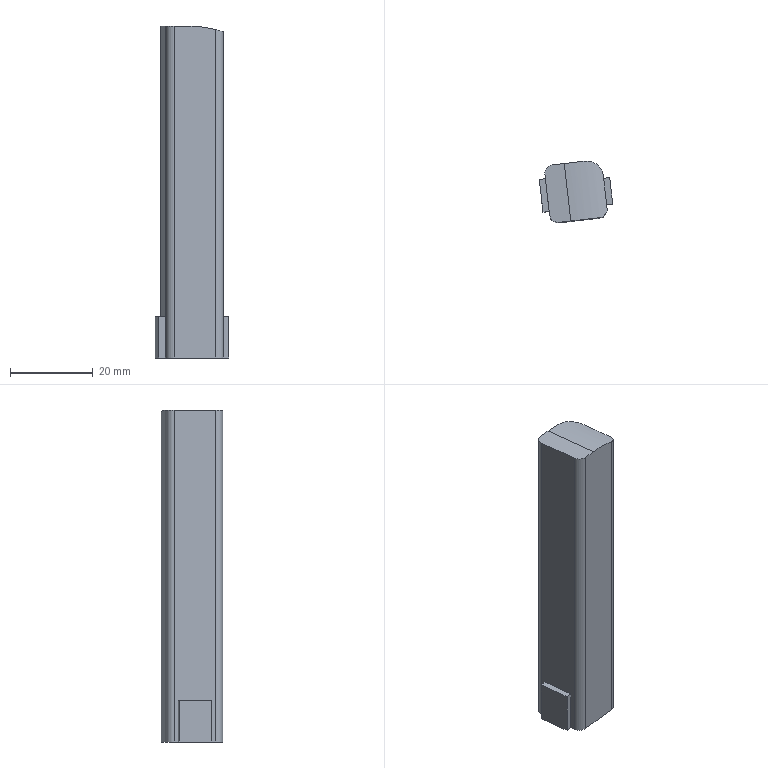Part | NX | features solid 2 | 1 solid | 19 faces | box 17.796 x 14.854 x 80.4 mm | volume 15437 mm3 | plane 14 | cylinder 5 | commonest cylinder face diameters 4 x3 8 x1 59 x1
STEP:
#1=CARTESIAN_POINT('',(2069.672,191.776,-68.));
#2=VERTEX_POINT('',#1);
#3=CARTESIAN_POINT('',(2070.408,185.318,-68.));
#4=VERTEX_POINT('',#3);
#5=CARTESIAN_POINT('',(2069.955,189.292,-68.));
#6=DIRECTION('',(0.1132,-0.9936,0.));
#7=VECTOR('',#6,1000.);
#8=LINE('',#5,#7);
#9=EDGE_CURVE('',#2,#4,#8,.T.);
#10=ORIENTED_EDGE('',*,*,#9,.F.);
#11=CARTESIAN_POINT('',(2069.672,191.776,-78.));
#12=VERTEX_POINT('',#11);
#13=CARTESIAN_POINT('',(2069.672,191.776,-63.));
#14=DIRECTION('',(0.,0.,-1.));
#15=VECTOR('',#14,1000.);
#16=LINE('',#13,#15);
#17=EDGE_CURVE('',#2,#12,#16,.T.);
#18=ORIENTED_EDGE('',*,*,#17,.T.);
#19=CARTESIAN_POINT('',(2069.615,192.273,-78.));
#20=VERTEX_POINT('',#19);
#21=CARTESIAN_POINT('',(2069.955,189.292,-78.));
#22=DIRECTION('',(0.1132,-0.9936,0.));
#23=VECTOR('',#22,1000.);
#24=LINE('',#21,#23);
#25=EDGE_CURVE('',#20,#12,#24,.T.);
#26=ORIENTED_EDGE('',*,*,#25,.F.);
#27=CARTESIAN_POINT('',(2069.615,192.273,0.9709));
#28=VERTEX_POINT('',#27);
#29=CARTESIAN_POINT('',(2069.615,192.273,-63.));
#30=DIRECTION('',(0.,0.,-1.));
#31=VECTOR('',#30,1000.);
#32=LINE('',#29,#31);
#33=EDGE_CURVE('',#28,#20,#32,.T.);
#34=ORIENTED_EDGE('',*,*,#33,.F.);
#35=CARTESIAN_POINT('',(2070.521,184.325,0.9709));
#36=VERTEX_POINT('',#35);
#37=CARTESIAN_POINT('',(2070.521,184.325,0.9709));
#38=CARTESIAN_POINT('',(2070.219,186.974,0.9709));
#39=CARTESIAN_POINT('',(2069.917,189.624,0.9709));
#40=CARTESIAN_POINT('',(2069.615,192.273,0.9709));
#41=B_SPLINE_CURVE_WITH_KNOTS('',3,(#37,#38,#39,#40),.UNSPECIFIED.,.F.,.F.,(4,4),(0.,1.),.PIECEWISE_BEZIER_KNOTS.);
#42=EDGE_CURVE('',#36,#28,#41,.T.);
#43=ORIENTED_EDGE('',*,*,#42,.F.);
#44=CARTESIAN_POINT('',(2070.521,184.325,-78.));
#45=VERTEX_POINT('',#44);
#46=CARTESIAN_POINT('',(2070.521,184.325,-63.));
#47=DIRECTION('',(0.,0.,-1.));
#48=VECTOR('',#47,1000.);
#49=LINE('',#46,#48);
#50=EDGE_CURVE('',#36,#45,#49,.T.);
#51=ORIENTED_EDGE('',*,*,#50,.T.);
#52=CARTESIAN_POINT('',(2070.408,185.318,-78.));
#53=VERTEX_POINT('',#52);
#54=CARTESIAN_POINT('',(2069.955,189.292,-78.));
#55=DIRECTION('',(0.1132,-0.9936,0.));
#56=VECTOR('',#55,1000.);
#57=LINE('',#54,#56);
#58=EDGE_CURVE('',#53,#45,#57,.T.);
#59=ORIENTED_EDGE('',*,*,#58,.F.);
#60=CARTESIAN_POINT('',(2070.408,185.318,-63.));
#61=DIRECTION('',(0.,0.,-1.));
#62=VECTOR('',#61,1000.);
#63=LINE('',#60,#62);
#64=EDGE_CURVE('',#4,#53,#63,.T.);
#65=ORIENTED_EDGE('',*,*,#64,.F.);
#66=EDGE_LOOP('',(#10,#18,#26,#34,#43,#51,#59,#65));
#67=FACE_BOUND('',#66,.T.);
#68=CARTESIAN_POINT('',(2069.955,189.292,-63.));
#69=DIRECTION('',(0.9936,0.1132,0.));
#70=DIRECTION('',(0.,0.,1.));
#71=AXIS2_PLACEMENT_3D('',#68,#69,#70);
#72=PLANE('',#71);
#73=ADVANCED_FACE('',(#67),#72,.T.);
#74=CARTESIAN_POINT('',(2056.498,183.733,-68.));
#75=VERTEX_POINT('',#74);
#76=CARTESIAN_POINT('',(2055.592,191.682,-68.));
#77=VERTEX_POINT('',#76);
#78=CARTESIAN_POINT('',(2056.045,187.708,-68.));
#79=DIRECTION('',(-0.1132,0.9936,0.));
#80=VECTOR('',#79,1000.);
#81=LINE('',#78,#80);
#82=EDGE_CURVE('',#75,#77,#81,.T.);
#83=ORIENTED_EDGE('',*,*,#82,.F.);
#84=CARTESIAN_POINT('',(2056.498,183.733,-78.));
#85=VERTEX_POINT('',#84);
#86=CARTESIAN_POINT('',(2056.498,183.733,-63.));
#87=DIRECTION('',(0.,0.,-1.));
#88=VECTOR('',#87,1000.);
#89=LINE('',#86,#88);
#90=EDGE_CURVE('',#75,#85,#89,.T.);
#91=ORIENTED_EDGE('',*,*,#90,.T.);
#92=CARTESIAN_POINT('',(2056.611,182.74,-78.));
#93=VERTEX_POINT('',#92);
#94=CARTESIAN_POINT('',(2056.045,187.708,-78.));
#95=DIRECTION('',(-0.1132,0.9936,0.));
#96=VECTOR('',#95,1000.);
#97=LINE('',#94,#96);
#98=EDGE_CURVE('',#93,#85,#97,.T.);
#99=ORIENTED_EDGE('',*,*,#98,.F.);
#100=CARTESIAN_POINT('',(2056.611,182.74,2.4));
#101=VERTEX_POINT('',#100);
#102=CARTESIAN_POINT('',(2056.611,182.74,-63.));
#103=DIRECTION('',(0.,0.,-1.));
#104=VECTOR('',#103,1000.);
#105=LINE('',#102,#104);
#106=EDGE_CURVE('',#101,#93,#105,.T.);
#107=ORIENTED_EDGE('',*,*,#106,.F.);
#108=CARTESIAN_POINT('',(2055.479,192.675,2.4));
#109=VERTEX_POINT('',#108);
#110=CARTESIAN_POINT('',(1900.081,1556.526,2.4));
#111=DIRECTION('',(0.1132,-0.9936,0.000000004));
#112=VECTOR('',#111,1000.);
#113=LINE('',#110,#112);
#114=EDGE_CURVE('',#109,#101,#113,.T.);
#115=ORIENTED_EDGE('',*,*,#114,.F.);
#116=CARTESIAN_POINT('',(2055.479,192.675,-78.));
#117=VERTEX_POINT('',#116);
#118=CARTESIAN_POINT('',(2055.479,192.675,-63.));
#119=DIRECTION('',(0.,0.,-1.));
#120=VECTOR('',#119,1000.);
#121=LINE('',#118,#120);
#122=EDGE_CURVE('',#109,#117,#121,.T.);
#123=ORIENTED_EDGE('',*,*,#122,.T.);
#124=CARTESIAN_POINT('',(2055.592,191.682,-78.));
#125=VERTEX_POINT('',#124);
#126=CARTESIAN_POINT('',(2056.045,187.708,-78.));
#127=DIRECTION('',(-0.1132,0.9936,0.));
#128=VECTOR('',#127,1000.);
#129=LINE('',#126,#128);
#130=EDGE_CURVE('',#125,#117,#129,.T.);
#131=ORIENTED_EDGE('',*,*,#130,.F.);
#132=CARTESIAN_POINT('',(2055.592,191.682,-63.));
#133=DIRECTION('',(0.,0.,-1.));
#134=VECTOR('',#133,1000.);
#135=LINE('',#132,#134);
#136=EDGE_CURVE('',#77,#125,#135,.T.);
#137=ORIENTED_EDGE('',*,*,#136,.F.);
#138=EDGE_LOOP('',(#83,#91,#99,#107,#115,#123,#131,#137));
#139=FACE_BOUND('',#138,.T.);
#140=CARTESIAN_POINT('',(2056.045,187.708,-63.));
#141=DIRECTION('',(-0.9936,-0.1132,0.));
#142=DIRECTION('',(0.,0.,-1.));
#143=AXIS2_PLACEMENT_3D('',#140,#141,#142);
#144=PLANE('',#143);
#145=ADVANCED_FACE('',(#139),#144,.T.);
#146=CARTESIAN_POINT('',(2058.825,180.979,2.4));
#147=VERTEX_POINT('',#146);
#148=CARTESIAN_POINT('',(2058.825,180.979,-78.));
#149=VERTEX_POINT('',#148);
#150=CARTESIAN_POINT('',(2058.825,180.979,-63.));
#151=DIRECTION('',(0.,0.,-1.));
#152=VECTOR('',#151,1000.);
#153=LINE('',#150,#152);
#154=EDGE_CURVE('',#147,#149,#153,.T.);
#155=ORIENTED_EDGE('',*,*,#154,.T.);
#156=CARTESIAN_POINT('',(2068.76,182.111,-78.));
#157=VERTEX_POINT('',#156);
#158=CARTESIAN_POINT('',(2063.792,181.545,-78.));
#159=DIRECTION('',(0.9936,0.1132,0.));
#160=VECTOR('',#159,1000.);
#161=LINE('',#158,#160);
#162=EDGE_CURVE('',#149,#157,#161,.T.);
#163=ORIENTED_EDGE('',*,*,#162,.T.);
#164=CARTESIAN_POINT('',(2068.76,182.111,1.54));
#165=VERTEX_POINT('',#164);
#166=CARTESIAN_POINT('',(2068.76,182.111,-63.));
#167=DIRECTION('',(0.,0.,-1.));
#168=VECTOR('',#167,1000.);
#169=LINE('',#166,#168);
#170=EDGE_CURVE('',#165,#157,#169,.T.);
#171=ORIENTED_EDGE('',*,*,#170,.F.);
#172=CARTESIAN_POINT('',(2061.735,181.311,2.4));
#173=VERTEX_POINT('',#172);
#174=CARTESIAN_POINT('',(2061.735,181.311,-27.1));
#175=DIRECTION('',(-0.1132,0.9936,0.));
#176=DIRECTION('',(-0.9936,-0.1132,0.00081));
#177=AXIS2_PLACEMENT_3D('',#174,#175,#176);
#178=ELLIPSE('',#177,29.5,29.5);
#179=EDGE_CURVE('',#173,#165,#178,.T.);
#180=ORIENTED_EDGE('',*,*,#179,.F.);
#181=CARTESIAN_POINT('',(1280.574,92.305,2.4));
#182=DIRECTION('',(0.9936,0.1132,-0.000000001));
#183=VECTOR('',#182,1000.);
#184=LINE('',#181,#183);
#185=EDGE_CURVE('',#147,#173,#184,.T.);
#186=ORIENTED_EDGE('',*,*,#185,.F.);
#187=EDGE_LOOP('',(#155,#163,#171,#180,#186));
#188=FACE_BOUND('',#187,.T.);
#189=CARTESIAN_POINT('',(2063.792,181.545,-63.));
#190=DIRECTION('',(0.1132,-0.9936,0.));
#191=DIRECTION('',(0.,0.,1.));
#192=AXIS2_PLACEMENT_3D('',#189,#190,#191);
#193=PLANE('',#192);
#194=ADVANCED_FACE('',(#188),#193,.T.);
#195=CARTESIAN_POINT('',(2065.188,195.795,1.961));
#196=VERTEX_POINT('',#195);
#197=CARTESIAN_POINT('',(2065.188,195.795,-78.));
#198=VERTEX_POINT('',#197);
#199=CARTESIAN_POINT('',(2065.188,195.795,-63.));
#200=DIRECTION('',(0.,0.,-1.));
#201=VECTOR('',#200,1000.);
#202=LINE('',#199,#201);
#203=EDGE_CURVE('',#196,#198,#202,.T.);
#204=ORIENTED_EDGE('',*,*,#203,.T.);
#205=CARTESIAN_POINT('',(2057.24,194.889,-78.));
#206=VERTEX_POINT('',#205);
#207=CARTESIAN_POINT('',(2062.208,195.455,-78.));
#208=DIRECTION('',(-0.9936,-0.1132,0.));
#209=VECTOR('',#208,1000.);
#210=LINE('',#207,#209);
#211=EDGE_CURVE('',#198,#206,#210,.T.);
#212=ORIENTED_EDGE('',*,*,#211,.T.);
#213=CARTESIAN_POINT('',(2057.24,194.889,2.4));
#214=VERTEX_POINT('',#213);
#215=CARTESIAN_POINT('',(2057.24,194.889,-63.));
#216=DIRECTION('',(0.,0.,-1.));
#217=VECTOR('',#216,1000.);
#218=LINE('',#215,#217);
#219=EDGE_CURVE('',#214,#206,#218,.T.);
#220=ORIENTED_EDGE('',*,*,#219,.F.);
#221=CARTESIAN_POINT('',(2060.15,195.221,2.4));
#222=VERTEX_POINT('',#221);
#223=CARTESIAN_POINT('',(1278.989,106.215,2.4));
#224=DIRECTION('',(0.9936,0.1132,-0.000000001));
#225=VECTOR('',#224,1000.);
#226=LINE('',#223,#225);
#227=EDGE_CURVE('',#214,#222,#226,.T.);
#228=ORIENTED_EDGE('',*,*,#227,.T.);
#229=CARTESIAN_POINT('',(2060.15,195.221,-27.1));
#230=DIRECTION('',(-0.1132,0.9936,0.));
#231=DIRECTION('',(-0.9936,-0.1132,0.00081));
#232=AXIS2_PLACEMENT_3D('',#229,#230,#231);
#233=ELLIPSE('',#232,29.5,29.5);
#234=EDGE_CURVE('',#222,#196,#233,.T.);
#235=ORIENTED_EDGE('',*,*,#234,.T.);
#236=EDGE_LOOP('',(#204,#212,#220,#228,#235));
#237=FACE_BOUND('',#236,.T.);
#238=CARTESIAN_POINT('',(2062.208,195.455,-63.));
#239=DIRECTION('',(-0.1132,0.9936,0.));
#240=DIRECTION('',(0.,0.,-1.));
#241=AXIS2_PLACEMENT_3D('',#238,#239,#240);
#242=PLANE('',#241);
#243=ADVANCED_FACE('',(#237),#242,.T.);
#244=CARTESIAN_POINT('',(2058.598,182.966,-78.));
#245=DIRECTION('',(0.,0.,-1.));
#246=DIRECTION('',(-1.,0.,0.));
#247=AXIS2_PLACEMENT_3D('',#244,#245,#246);
#248=CIRCLE('',#247,2.);
#249=EDGE_CURVE('',#149,#93,#248,.T.);
#250=ORIENTED_EDGE('',*,*,#249,.F.);
#251=ORIENTED_EDGE('',*,*,#154,.F.);
#252=CARTESIAN_POINT('',(2058.598,182.966,2.4));
#253=DIRECTION('',(0.,-0.000000004,-1.));
#254=DIRECTION('',(0.,1.,-0.000000004));
#255=AXIS2_PLACEMENT_3D('',#252,#253,#254);
#256=CIRCLE('',#255,2.);
#257=EDGE_CURVE('',#147,#101,#256,.T.);
#258=ORIENTED_EDGE('',*,*,#257,.T.);
#259=ORIENTED_EDGE('',*,*,#106,.T.);
#260=EDGE_LOOP('',(#250,#251,#258,#259));
#261=FACE_BOUND('',#260,.T.);
#262=CARTESIAN_POINT('',(2058.598,182.966,-63.));
#263=DIRECTION('',(0.,0.,1.));
#264=DIRECTION('',(-0.9936,-0.1132,0.));
#265=AXIS2_PLACEMENT_3D('',#262,#263,#264);
#266=CYLINDRICAL_SURFACE('',#265,2.);
#267=ADVANCED_FACE('',(#261),#266,.T.);
#268=CARTESIAN_POINT('',(2068.534,184.098,-78.));
#269=DIRECTION('',(0.,0.,-1.));
#270=DIRECTION('',(-1.,0.,0.));
#271=AXIS2_PLACEMENT_3D('',#268,#269,#270);
#272=CIRCLE('',#271,2.);
#273=EDGE_CURVE('',#45,#157,#272,.T.);
#274=ORIENTED_EDGE('',*,*,#273,.F.);
#275=ORIENTED_EDGE('',*,*,#50,.F.);
#276=CARTESIAN_POINT('',(2070.521,184.325,0.9709));
#277=CARTESIAN_POINT('',(2070.643,183.254,0.9709));
#278=CARTESIAN_POINT('',(2069.798,182.229,1.282));
#279=CARTESIAN_POINT('',(2068.76,182.111,1.54));
#280=B_SPLINE_CURVE_WITH_KNOTS('',3,(#276,#277,#278,#279),.UNSPECIFIED.,.F.,.F.,(4,4),(0.,0.003185),.UNSPECIFIED.);
#281=EDGE_CURVE('',#36,#165,#280,.T.);
#282=ORIENTED_EDGE('',*,*,#281,.T.);
#283=ORIENTED_EDGE('',*,*,#170,.T.);
#284=EDGE_LOOP('',(#274,#275,#282,#283));
#285=FACE_BOUND('',#284,.T.);
#286=CARTESIAN_POINT('',(2068.534,184.098,-63.));
#287=DIRECTION('',(0.,0.,1.));
#288=DIRECTION('',(-0.9936,-0.1132,0.));
#289=AXIS2_PLACEMENT_3D('',#286,#287,#288);
#290=CYLINDRICAL_SURFACE('',#289,2.);
#291=ADVANCED_FACE('',(#285),#290,.T.);
#292=CARTESIAN_POINT('',(2065.641,191.82,-78.));
#293=DIRECTION('',(0.,0.,-1.));
#294=DIRECTION('',(-1.,0.,0.));
#295=AXIS2_PLACEMENT_3D('',#292,#293,#294);
#296=CIRCLE('',#295,4.);
#297=EDGE_CURVE('',#198,#20,#296,.T.);
#298=ORIENTED_EDGE('',*,*,#297,.F.);
#299=ORIENTED_EDGE('',*,*,#203,.F.);
#300=CARTESIAN_POINT('',(2069.615,192.273,0.9709));
#301=CARTESIAN_POINT('',(2069.494,193.338,0.9709));
#302=CARTESIAN_POINT('',(2068.368,195.298,1.279));
#303=CARTESIAN_POINT('',(2066.237,195.914,1.777));
#304=CARTESIAN_POINT('',(2065.188,195.795,1.961));
#305=B_SPLINE_CURVE_WITH_KNOTS('',3,(#300,#301,#302,#303,#304),.UNSPECIFIED.,.F.,.F.,(4,1,4),(0.,0.003169,0.006337),.UNSPECIFIED.);
#306=EDGE_CURVE('',#28,#196,#305,.T.);
#307=ORIENTED_EDGE('',*,*,#306,.F.);
#308=ORIENTED_EDGE('',*,*,#33,.T.);
#309=EDGE_LOOP('',(#298,#299,#307,#308));
#310=FACE_BOUND('',#309,.T.);
#311=CARTESIAN_POINT('',(2065.641,191.82,-63.));
#312=DIRECTION('',(0.,0.,-1.));
#313=DIRECTION('',(1.,0.,0.));
#314=AXIS2_PLACEMENT_3D('',#311,#312,#313);
#315=CYLINDRICAL_SURFACE('',#314,4.);
#316=ADVANCED_FACE('',(#310),#315,.T.);
#317=CARTESIAN_POINT('',(2057.466,192.902,-78.));
#318=DIRECTION('',(0.,0.,-1.));
#319=DIRECTION('',(-1.,0.,0.));
#320=AXIS2_PLACEMENT_3D('',#317,#318,#319);
#321=CIRCLE('',#320,2.);
#322=EDGE_CURVE('',#117,#206,#321,.T.);
#323=ORIENTED_EDGE('',*,*,#322,.F.);
#324=ORIENTED_EDGE('',*,*,#122,.F.);
#325=CARTESIAN_POINT('',(2057.466,192.902,2.4));
#326=DIRECTION('',(0.,0.000000004,1.));
#327=DIRECTION('',(0.,1.,-0.000000004));
#328=AXIS2_PLACEMENT_3D('',#325,#326,#327);
#329=CIRCLE('',#328,2.);
#330=EDGE_CURVE('',#214,#109,#329,.T.);
#331=ORIENTED_EDGE('',*,*,#330,.F.);
#332=ORIENTED_EDGE('',*,*,#219,.T.);
#333=EDGE_LOOP('',(#323,#324,#331,#332));
#334=FACE_BOUND('',#333,.T.);
#335=CARTESIAN_POINT('',(2057.466,192.902,-63.));
#336=DIRECTION('',(0.,0.,1.));
#337=DIRECTION('',(-0.9936,-0.1132,0.));
#338=AXIS2_PLACEMENT_3D('',#335,#336,#337);
#339=CYLINDRICAL_SURFACE('',#338,2.);
#340=ADVANCED_FACE('',(#334),#339,.T.);
#341=ORIENTED_EDGE('',*,*,#297,.T.);
#342=ORIENTED_EDGE('',*,*,#25,.T.);
#343=CARTESIAN_POINT('',(2071.162,191.946,-78.));
#344=VERTEX_POINT('',#343);
#345=CARTESIAN_POINT('',(2070.666,191.89,-78.));
#346=DIRECTION('',(-0.9936,-0.1132,0.));
#347=VECTOR('',#346,1000.);
#348=LINE('',#345,#347);
#349=EDGE_CURVE('',#344,#12,#348,.T.);
#350=ORIENTED_EDGE('',*,*,#349,.F.);
#351=CARTESIAN_POINT('',(2071.898,185.488,-78.));
#352=VERTEX_POINT('',#351);
#353=CARTESIAN_POINT('',(2071.445,189.462,-78.));
#354=DIRECTION('',(0.1132,-0.9936,0.));
#355=VECTOR('',#354,1000.);
#356=LINE('',#353,#355);
#357=EDGE_CURVE('',#344,#352,#356,.T.);
#358=ORIENTED_EDGE('',*,*,#357,.T.);
#359=CARTESIAN_POINT('',(2071.401,185.431,-78.));
#360=DIRECTION('',(-0.9936,-0.1132,0.));
#361=VECTOR('',#360,1000.);
#362=LINE('',#359,#361);
#363=EDGE_CURVE('',#352,#53,#362,.T.);
#364=ORIENTED_EDGE('',*,*,#363,.T.);
#365=ORIENTED_EDGE('',*,*,#58,.T.);
#366=ORIENTED_EDGE('',*,*,#273,.T.);
#367=ORIENTED_EDGE('',*,*,#162,.F.);
#368=ORIENTED_EDGE('',*,*,#249,.T.);
#369=ORIENTED_EDGE('',*,*,#98,.T.);
#370=CARTESIAN_POINT('',(2055.007,183.563,-78.));
#371=VERTEX_POINT('',#370);
#372=CARTESIAN_POINT('',(2055.504,183.62,-78.));
#373=DIRECTION('',(0.9936,0.1132,0.));
#374=VECTOR('',#373,1000.);
#375=LINE('',#372,#374);
#376=EDGE_CURVE('',#371,#85,#375,.T.);
#377=ORIENTED_EDGE('',*,*,#376,.F.);
#378=CARTESIAN_POINT('',(2054.102,191.512,-78.));
#379=VERTEX_POINT('',#378);
#380=CARTESIAN_POINT('',(2054.555,187.538,-78.));
#381=DIRECTION('',(-0.1132,0.9936,0.));
#382=VECTOR('',#381,1000.);
#383=LINE('',#380,#382);
#384=EDGE_CURVE('',#371,#379,#383,.T.);
#385=ORIENTED_EDGE('',*,*,#384,.T.);
#386=CARTESIAN_POINT('',(2054.599,191.569,-78.));
#387=DIRECTION('',(0.9936,0.1132,0.));
#388=VECTOR('',#387,1000.);
#389=LINE('',#386,#388);
#390=EDGE_CURVE('',#379,#125,#389,.T.);
#391=ORIENTED_EDGE('',*,*,#390,.T.);
#392=ORIENTED_EDGE('',*,*,#130,.T.);
#393=ORIENTED_EDGE('',*,*,#322,.T.);
#394=ORIENTED_EDGE('',*,*,#211,.F.);
#395=EDGE_LOOP('',(#341,#342,#350,#358,#364,#365,#366,#367,#368,#369,#377,#385,#391,#392,#393,#394));
#396=FACE_BOUND('',#395,.T.);
#397=CARTESIAN_POINT('',(2063.,188.5,-78.));
#398=DIRECTION('',(0.,0.,-1.));
#399=DIRECTION('',(0.9936,0.1132,0.));
#400=AXIS2_PLACEMENT_3D('',#397,#398,#399);
#401=PLANE('',#400);
#402=ADVANCED_FACE('',(#396),#401,.T.);
#403=ORIENTED_EDGE('',*,*,#257,.F.);
#404=ORIENTED_EDGE('',*,*,#185,.T.);
#405=CARTESIAN_POINT('',(2060.943,188.266,2.4));
#406=DIRECTION('',(-0.1132,0.9936,-0.000000004));
#407=VECTOR('',#406,1000.);
#408=LINE('',#405,#407);
#409=EDGE_CURVE('',#173,#222,#408,.T.);
#410=ORIENTED_EDGE('',*,*,#409,.T.);
#411=ORIENTED_EDGE('',*,*,#227,.F.);
#412=ORIENTED_EDGE('',*,*,#330,.T.);
#413=ORIENTED_EDGE('',*,*,#114,.T.);
#414=EDGE_LOOP('',(#403,#404,#410,#411,#412,#413));
#415=FACE_BOUND('',#414,.T.);
#416=CARTESIAN_POINT('',(1123.818,1468.078,2.4));
#417=DIRECTION('',(0.,-0.000000004,-1.));
#418=DIRECTION('',(-0.09584,-0.9954,0.000000004));
#419=AXIS2_PLACEMENT_3D('',#416,#417,#418);
#420=PLANE('',#419);
#421=ADVANCED_FACE('',(#415),#420,.F.);
#422=ORIENTED_EDGE('',*,*,#179,.T.);
#423=ORIENTED_EDGE('',*,*,#281,.F.);
#424=ORIENTED_EDGE('',*,*,#42,.T.);
#425=ORIENTED_EDGE('',*,*,#306,.T.);
#426=ORIENTED_EDGE('',*,*,#234,.F.);
#427=ORIENTED_EDGE('',*,*,#409,.F.);
#428=EDGE_LOOP('',(#422,#423,#424,#425,#426,#427));
#429=FACE_BOUND('',#428,.T.);
#430=CARTESIAN_POINT('',(2060.632,190.994,-27.1));
#431=DIRECTION('',(0.1132,-0.9936,0.000000004));
#432=DIRECTION('',(-0.9936,-0.1132,0.000000001));
#433=AXIS2_PLACEMENT_3D('',#430,#431,#432);
#434=CYLINDRICAL_SURFACE('',#433,29.5);
#435=ADVANCED_FACE('',(#429),#434,.T.);
#436=ORIENTED_EDGE('',*,*,#90,.F.);
#437=CARTESIAN_POINT('',(2055.007,183.563,-68.));
#438=VERTEX_POINT('',#437);
#439=CARTESIAN_POINT('',(2055.504,183.62,-68.));
#440=DIRECTION('',(-0.9936,-0.1132,0.));
#441=VECTOR('',#440,1000.);
#442=LINE('',#439,#441);
#443=EDGE_CURVE('',#75,#438,#442,.T.);
#444=ORIENTED_EDGE('',*,*,#443,.T.);
#445=CARTESIAN_POINT('',(2055.007,183.563,-63.));
#446=DIRECTION('',(0.,0.,-1.));
#447=VECTOR('',#446,1000.);
#448=LINE('',#445,#447);
#449=EDGE_CURVE('',#438,#371,#448,.T.);
#450=ORIENTED_EDGE('',*,*,#449,.T.);
#451=ORIENTED_EDGE('',*,*,#376,.T.);
#452=EDGE_LOOP('',(#436,#444,#450,#451));
#453=FACE_BOUND('',#452,.T.);
#454=CARTESIAN_POINT('',(2055.504,183.62,-63.));
#455=DIRECTION('',(0.1132,-0.9936,0.));
#456=DIRECTION('',(-0.9936,-0.1132,0.));
#457=AXIS2_PLACEMENT_3D('',#454,#455,#456);
#458=PLANE('',#457);
#459=ADVANCED_FACE('',(#453),#458,.T.);
#460=CARTESIAN_POINT('',(2054.102,191.512,-68.));
#461=VERTEX_POINT('',#460);
#462=CARTESIAN_POINT('',(2054.599,191.569,-68.));
#463=DIRECTION('',(-0.9936,-0.1132,0.));
#464=VECTOR('',#463,1000.);
#465=LINE('',#462,#464);
#466=EDGE_CURVE('',#77,#461,#465,.T.);
#467=ORIENTED_EDGE('',*,*,#466,.F.);
#468=ORIENTED_EDGE('',*,*,#136,.T.);
#469=ORIENTED_EDGE('',*,*,#390,.F.);
#470=CARTESIAN_POINT('',(2054.102,191.512,-63.));
#471=DIRECTION('',(0.,0.,-1.));
#472=VECTOR('',#471,1000.);
#473=LINE('',#470,#472);
#474=EDGE_CURVE('',#461,#379,#473,.T.);
#475=ORIENTED_EDGE('',*,*,#474,.F.);
#476=EDGE_LOOP('',(#467,#468,#469,#475));
#477=FACE_BOUND('',#476,.T.);
#478=CARTESIAN_POINT('',(2054.599,191.569,-63.));
#479=DIRECTION('',(0.1132,-0.9936,0.));
#480=DIRECTION('',(-0.9936,-0.1132,0.));
#481=AXIS2_PLACEMENT_3D('',#478,#479,#480);
#482=PLANE('',#481);
#483=ADVANCED_FACE('',(#477),#482,.F.);
#484=ORIENTED_EDGE('',*,*,#449,.F.);
#485=CARTESIAN_POINT('',(2054.555,187.538,-68.));
#486=DIRECTION('',(-0.1132,0.9936,0.));
#487=VECTOR('',#486,1000.);
#488=LINE('',#485,#487);
#489=EDGE_CURVE('',#438,#461,#488,.T.);
#490=ORIENTED_EDGE('',*,*,#489,.T.);
#491=ORIENTED_EDGE('',*,*,#474,.T.);
#492=ORIENTED_EDGE('',*,*,#384,.F.);
#493=EDGE_LOOP('',(#484,#490,#491,#492));
#494=FACE_BOUND('',#493,.T.);
#495=CARTESIAN_POINT('',(2054.555,187.538,-63.));
#496=DIRECTION('',(-0.9936,-0.1132,0.));
#497=DIRECTION('',(0.,0.,-1.));
#498=AXIS2_PLACEMENT_3D('',#495,#496,#497);
#499=PLANE('',#498);
#500=ADVANCED_FACE('',(#494),#499,.T.);
#501=ORIENTED_EDGE('',*,*,#489,.F.);
#502=ORIENTED_EDGE('',*,*,#443,.F.);
#503=ORIENTED_EDGE('',*,*,#82,.T.);
#504=ORIENTED_EDGE('',*,*,#466,.T.);
#505=EDGE_LOOP('',(#501,#502,#503,#504));
#506=FACE_BOUND('',#505,.T.);
#507=CARTESIAN_POINT('',(2063.,188.393,-68.));
#508=DIRECTION('',(0.,0.,1.));
#509=DIRECTION('',(-1.,0.,0.));
#510=AXIS2_PLACEMENT_3D('',#507,#508,#509);
#511=PLANE('',#510);
#512=ADVANCED_FACE('',(#506),#511,.T.);
#513=ORIENTED_EDGE('',*,*,#17,.F.);
#514=CARTESIAN_POINT('',(2071.162,191.946,-68.));
#515=VERTEX_POINT('',#514);
#516=CARTESIAN_POINT('',(2070.666,191.89,-68.));
#517=DIRECTION('',(0.9936,0.1132,0.));
#518=VECTOR('',#517,1000.);
#519=LINE('',#516,#518);
#520=EDGE_CURVE('',#2,#515,#519,.T.);
#521=ORIENTED_EDGE('',*,*,#520,.T.);
#522=CARTESIAN_POINT('',(2071.162,191.946,-63.));
#523=DIRECTION('',(0.,0.,-1.));
#524=VECTOR('',#523,1000.);
#525=LINE('',#522,#524);
#526=EDGE_CURVE('',#515,#344,#525,.T.);
#527=ORIENTED_EDGE('',*,*,#526,.T.);
#528=ORIENTED_EDGE('',*,*,#349,.T.);
#529=EDGE_LOOP('',(#513,#521,#527,#528));
#530=FACE_BOUND('',#529,.T.);
#531=CARTESIAN_POINT('',(2070.666,191.89,-63.));
#532=DIRECTION('',(-0.1132,0.9936,0.));
#533=DIRECTION('',(0.9936,0.1132,0.));
#534=AXIS2_PLACEMENT_3D('',#531,#532,#533);
#535=PLANE('',#534);
#536=ADVANCED_FACE('',(#530),#535,.T.);
#537=CARTESIAN_POINT('',(2071.898,185.488,-68.));
#538=VERTEX_POINT('',#537);
#539=CARTESIAN_POINT('',(2071.401,185.431,-68.));
#540=DIRECTION('',(0.9936,0.1132,0.));
#541=VECTOR('',#540,1000.);
#542=LINE('',#539,#541);
#543=EDGE_CURVE('',#4,#538,#542,.T.);
#544=ORIENTED_EDGE('',*,*,#543,.F.);
#545=ORIENTED_EDGE('',*,*,#64,.T.);
#546=ORIENTED_EDGE('',*,*,#363,.F.);
#547=CARTESIAN_POINT('',(2071.898,185.488,-63.));
#548=DIRECTION('',(0.,0.,-1.));
#549=VECTOR('',#548,1000.);
#550=LINE('',#547,#549);
#551=EDGE_CURVE('',#538,#352,#550,.T.);
#552=ORIENTED_EDGE('',*,*,#551,.F.);
#553=EDGE_LOOP('',(#544,#545,#546,#552));
#554=FACE_BOUND('',#553,.T.);
#555=CARTESIAN_POINT('',(2071.401,185.431,-63.));
#556=DIRECTION('',(-0.1132,0.9936,0.));
#557=DIRECTION('',(0.9936,0.1132,0.));
#558=AXIS2_PLACEMENT_3D('',#555,#556,#557);
#559=PLANE('',#558);
#560=ADVANCED_FACE('',(#554),#559,.F.);
#561=ORIENTED_EDGE('',*,*,#526,.F.);
#562=CARTESIAN_POINT('',(2071.445,189.462,-68.));
#563=DIRECTION('',(0.1132,-0.9936,0.));
#564=VECTOR('',#563,1000.);
#565=LINE('',#562,#564);
#566=EDGE_CURVE('',#515,#538,#565,.T.);
#567=ORIENTED_EDGE('',*,*,#566,.T.);
#568=ORIENTED_EDGE('',*,*,#551,.T.);
#569=ORIENTED_EDGE('',*,*,#357,.F.);
#570=EDGE_LOOP('',(#561,#567,#568,#569));
#571=FACE_BOUND('',#570,.T.);
#572=CARTESIAN_POINT('',(2071.445,189.462,-63.));
#573=DIRECTION('',(0.9936,0.1132,0.));
#574=DIRECTION('',(0.,0.,1.));
#575=AXIS2_PLACEMENT_3D('',#572,#573,#574);
#576=PLANE('',#575);
#577=ADVANCED_FACE('',(#571),#576,.T.);
#578=ORIENTED_EDGE('',*,*,#566,.F.);
#579=ORIENTED_EDGE('',*,*,#520,.F.);
#580=ORIENTED_EDGE('',*,*,#9,.T.);
#581=ORIENTED_EDGE('',*,*,#543,.T.);
#582=EDGE_LOOP('',(#578,#579,#580,#581));
#583=FACE_BOUND('',#582,.T.);
#584=CARTESIAN_POINT('',(2063.,188.393,-68.));
#585=DIRECTION('',(0.,0.,1.));
#586=DIRECTION('',(-1.,0.,0.));
#587=AXIS2_PLACEMENT_3D('',#584,#585,#586);
#588=PLANE('',#587);
#589=ADVANCED_FACE('',(#583),#588,.T.);
#590=CLOSED_SHELL('',(#73,#145,#194,#243,#267,#291,#316,#340,#402,#421,#435,#459,#483,#500,#512,#536,#560,#577,#589));
#591=MANIFOLD_SOLID_BREP('',#590);
#592=(LENGTH_UNIT()NAMED_UNIT(*)SI_UNIT(.MILLI.,.METRE.));
#593=UNCERTAINTY_MEASURE_WITH_UNIT(LENGTH_MEASURE(0.0508),#592,'','');
#594=(NAMED_UNIT(*)PLANE_ANGLE_UNIT()SI_UNIT($,.RADIAN.));
#595=(NAMED_UNIT(*)SI_UNIT($,.STERADIAN.)SOLID_ANGLE_UNIT());
#596=(GEOMETRIC_REPRESENTATION_CONTEXT(3)GLOBAL_UNCERTAINTY_ASSIGNED_CONTEXT((#593))GLOBAL_UNIT_ASSIGNED_CONTEXT((#592,#594,#595))REPRESENTATION_CONTEXT('',''));
#597=ADVANCED_BREP_SHAPE_REPRESENTATION('',(#591),#596);